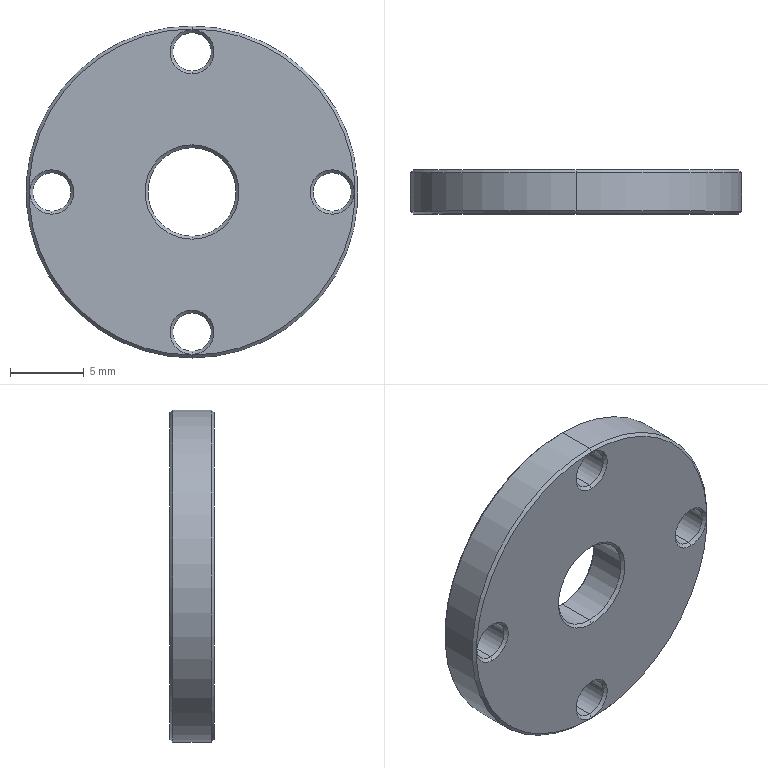Part | SolidWorks | features Chamfer 1, Extrusion 1 | 1 solid | 38 faces | box 22.5 x 3 x 22.5 mm | volume 1039 mm3 | cone 24 | cylinder 12 | plane 2 | commonest cylinder face diameters 2.6 x8 6 x2 22.5 x2
STEP:
#1=CARTESIAN_POINT('',(0.,2.8,8.2));
#2=VERTEX_POINT('',#1);
#3=CARTESIAN_POINT('',(0.,2.8,10.8));
#4=VERTEX_POINT('',#3);
#5=CARTESIAN_POINT('',(0.,2.8,9.5));
#6=DIRECTION('',(0.,1.,0.));
#7=DIRECTION('',(0.,0.,1.));
#8=AXIS2_PLACEMENT_3D('',#5,#6,#7);
#9=CIRCLE('',#8,1.3);
#10=EDGE_CURVE('',#2,#4,#9,.T.);
#11=ORIENTED_EDGE('',*,*,#10,.F.);
#12=CARTESIAN_POINT('',(0.,3.,8.));
#13=VERTEX_POINT('',#12);
#14=CARTESIAN_POINT('',(0.,2.8,8.2));
#15=DIRECTION('',(0.,0.7071,-0.7071));
#16=VECTOR('',#15,1000.);
#17=LINE('',#14,#16);
#18=EDGE_CURVE('',#2,#13,#17,.T.);
#19=ORIENTED_EDGE('',*,*,#18,.T.);
#20=CARTESIAN_POINT('',(0.,3.,11.));
#21=VERTEX_POINT('',#20);
#22=CARTESIAN_POINT('',(0.,3.,9.5));
#23=DIRECTION('',(0.,-1.,0.));
#24=DIRECTION('',(0.,0.,1.));
#25=AXIS2_PLACEMENT_3D('',#22,#23,#24);
#26=CIRCLE('',#25,1.5);
#27=EDGE_CURVE('',#21,#13,#26,.T.);
#28=ORIENTED_EDGE('',*,*,#27,.F.);
#29=CARTESIAN_POINT('',(0.,2.8,10.8));
#30=DIRECTION('',(0.,0.7071,0.7071));
#31=VECTOR('',#30,1000.);
#32=LINE('',#29,#31);
#33=EDGE_CURVE('',#4,#21,#32,.T.);
#34=ORIENTED_EDGE('',*,*,#33,.F.);
#35=EDGE_LOOP('',(#11,#19,#28,#34));
#36=FACE_OUTER_BOUND('',#35,.T.);
#37=CARTESIAN_POINT('',(0.,2.8,9.5));
#38=DIRECTION('',(0.,1.,0.));
#39=DIRECTION('',(0.,0.,1.));
#40=AXIS2_PLACEMENT_3D('',#37,#38,#39);
#41=CONICAL_SURFACE('',#40,1.3,0.7854);
#42=ADVANCED_FACE('',(#36),#41,.F.);
#43=CARTESIAN_POINT('',(0.,2.8,-3.));
#44=VERTEX_POINT('',#43);
#45=CARTESIAN_POINT('',(0.,2.8,3.));
#46=VERTEX_POINT('',#45);
#47=CARTESIAN_POINT('',(0.,2.8,0.));
#48=DIRECTION('',(0.,1.,0.));
#49=DIRECTION('',(0.,0.,1.));
#50=AXIS2_PLACEMENT_3D('',#47,#48,#49);
#51=CIRCLE('',#50,3.);
#52=EDGE_CURVE('',#44,#46,#51,.T.);
#53=ORIENTED_EDGE('',*,*,#52,.F.);
#54=CARTESIAN_POINT('',(0.,3.,-3.2));
#55=VERTEX_POINT('',#54);
#56=CARTESIAN_POINT('',(0.,2.8,-3.));
#57=DIRECTION('',(0.,0.7071,-0.7071));
#58=VECTOR('',#57,1000.);
#59=LINE('',#56,#58);
#60=EDGE_CURVE('',#44,#55,#59,.T.);
#61=ORIENTED_EDGE('',*,*,#60,.T.);
#62=CARTESIAN_POINT('',(0.,3.,3.2));
#63=VERTEX_POINT('',#62);
#64=CARTESIAN_POINT('',(0.,3.,0.));
#65=DIRECTION('',(0.,-1.,0.));
#66=DIRECTION('',(0.,0.,1.));
#67=AXIS2_PLACEMENT_3D('',#64,#65,#66);
#68=CIRCLE('',#67,3.2);
#69=EDGE_CURVE('',#63,#55,#68,.T.);
#70=ORIENTED_EDGE('',*,*,#69,.F.);
#71=CARTESIAN_POINT('',(0.,2.8,3.));
#72=DIRECTION('',(0.,0.7071,0.7071));
#73=VECTOR('',#72,1000.);
#74=LINE('',#71,#73);
#75=EDGE_CURVE('',#46,#63,#74,.T.);
#76=ORIENTED_EDGE('',*,*,#75,.F.);
#77=EDGE_LOOP('',(#53,#61,#70,#76));
#78=FACE_OUTER_BOUND('',#77,.T.);
#79=CARTESIAN_POINT('',(0.,2.8,0.));
#80=DIRECTION('',(0.,1.,0.));
#81=DIRECTION('',(0.,0.,1.));
#82=AXIS2_PLACEMENT_3D('',#79,#80,#81);
#83=CONICAL_SURFACE('',#82,3.,0.7854);
#84=ADVANCED_FACE('',(#78),#83,.F.);
#85=CARTESIAN_POINT('',(0.,3.,11.05));
#86=VERTEX_POINT('',#85);
#87=CARTESIAN_POINT('',(0.,3.,-11.05));
#88=VERTEX_POINT('',#87);
#89=CARTESIAN_POINT('',(0.,3.,0.));
#90=DIRECTION('',(0.,1.,0.));
#91=DIRECTION('',(0.,0.,1.));
#92=AXIS2_PLACEMENT_3D('',#89,#90,#91);
#93=CIRCLE('',#92,11.05);
#94=EDGE_CURVE('',#86,#88,#93,.T.);
#95=ORIENTED_EDGE('',*,*,#94,.F.);
#96=CARTESIAN_POINT('',(0.,2.8,11.25));
#97=VERTEX_POINT('',#96);
#98=CARTESIAN_POINT('',(0.,3.,11.05));
#99=DIRECTION('',(0.,-0.7071,0.7071));
#100=VECTOR('',#99,1000.);
#101=LINE('',#98,#100);
#102=EDGE_CURVE('',#86,#97,#101,.T.);
#103=ORIENTED_EDGE('',*,*,#102,.T.);
#104=CARTESIAN_POINT('',(0.,2.8,-11.25));
#105=VERTEX_POINT('',#104);
#106=CARTESIAN_POINT('',(0.,2.8,0.));
#107=DIRECTION('',(0.,-1.,0.));
#108=DIRECTION('',(0.,0.,1.));
#109=AXIS2_PLACEMENT_3D('',#106,#107,#108);
#110=CIRCLE('',#109,11.25);
#111=EDGE_CURVE('',#105,#97,#110,.T.);
#112=ORIENTED_EDGE('',*,*,#111,.F.);
#113=CARTESIAN_POINT('',(0.,3.,-11.05));
#114=DIRECTION('',(0.,-0.7071,-0.7071));
#115=VECTOR('',#114,1000.);
#116=LINE('',#113,#115);
#117=EDGE_CURVE('',#88,#105,#116,.T.);
#118=ORIENTED_EDGE('',*,*,#117,.F.);
#119=EDGE_LOOP('',(#95,#103,#112,#118));
#120=FACE_OUTER_BOUND('',#119,.T.);
#121=CARTESIAN_POINT('',(0.,3.,0.));
#122=DIRECTION('',(0.,-1.,0.));
#123=DIRECTION('',(0.,0.,-1.));
#124=AXIS2_PLACEMENT_3D('',#121,#122,#123);
#125=CONICAL_SURFACE('',#124,11.05,0.7854);
#126=ADVANCED_FACE('',(#120),#125,.T.);
#127=CARTESIAN_POINT('',(0.,2.8,-10.8));
#128=VERTEX_POINT('',#127);
#129=CARTESIAN_POINT('',(0.,2.8,-8.2));
#130=VERTEX_POINT('',#129);
#131=CARTESIAN_POINT('',(0.,2.8,-9.5));
#132=DIRECTION('',(0.,1.,0.));
#133=DIRECTION('',(0.,0.,1.));
#134=AXIS2_PLACEMENT_3D('',#131,#132,#133);
#135=CIRCLE('',#134,1.3);
#136=EDGE_CURVE('',#128,#130,#135,.T.);
#137=ORIENTED_EDGE('',*,*,#136,.F.);
#138=CARTESIAN_POINT('',(0.,3.,-11.));
#139=VERTEX_POINT('',#138);
#140=CARTESIAN_POINT('',(0.,2.8,-10.8));
#141=DIRECTION('',(0.,0.7071,-0.7071));
#142=VECTOR('',#141,1000.);
#143=LINE('',#140,#142);
#144=EDGE_CURVE('',#128,#139,#143,.T.);
#145=ORIENTED_EDGE('',*,*,#144,.T.);
#146=CARTESIAN_POINT('',(0.,3.,-8.));
#147=VERTEX_POINT('',#146);
#148=CARTESIAN_POINT('',(0.,3.,-9.5));
#149=DIRECTION('',(0.,-1.,0.));
#150=DIRECTION('',(0.,0.,1.));
#151=AXIS2_PLACEMENT_3D('',#148,#149,#150);
#152=CIRCLE('',#151,1.5);
#153=EDGE_CURVE('',#147,#139,#152,.T.);
#154=ORIENTED_EDGE('',*,*,#153,.F.);
#155=CARTESIAN_POINT('',(0.,2.8,-8.2));
#156=DIRECTION('',(0.,0.7071,0.7071));
#157=VECTOR('',#156,1000.);
#158=LINE('',#155,#157);
#159=EDGE_CURVE('',#130,#147,#158,.T.);
#160=ORIENTED_EDGE('',*,*,#159,.F.);
#161=EDGE_LOOP('',(#137,#145,#154,#160));
#162=FACE_OUTER_BOUND('',#161,.T.);
#163=CARTESIAN_POINT('',(0.,2.8,-9.5));
#164=DIRECTION('',(0.,1.,0.));
#165=DIRECTION('',(0.,0.,1.));
#166=AXIS2_PLACEMENT_3D('',#163,#164,#165);
#167=CONICAL_SURFACE('',#166,1.3,0.7854);
#168=ADVANCED_FACE('',(#162),#167,.F.);
#169=CARTESIAN_POINT('',(9.5,2.8,-1.3));
#170=VERTEX_POINT('',#169);
#171=CARTESIAN_POINT('',(9.5,2.8,1.3));
#172=VERTEX_POINT('',#171);
#173=CARTESIAN_POINT('',(9.5,2.8,0.));
#174=DIRECTION('',(0.,1.,0.));
#175=DIRECTION('',(0.,0.,1.));
#176=AXIS2_PLACEMENT_3D('',#173,#174,#175);
#177=CIRCLE('',#176,1.3);
#178=EDGE_CURVE('',#170,#172,#177,.T.);
#179=ORIENTED_EDGE('',*,*,#178,.F.);
#180=CARTESIAN_POINT('',(9.5,3.,-1.5));
#181=VERTEX_POINT('',#180);
#182=CARTESIAN_POINT('',(9.5,2.8,-1.3));
#183=DIRECTION('',(0.,0.7071,-0.7071));
#184=VECTOR('',#183,1000.);
#185=LINE('',#182,#184);
#186=EDGE_CURVE('',#170,#181,#185,.T.);
#187=ORIENTED_EDGE('',*,*,#186,.T.);
#188=CARTESIAN_POINT('',(9.5,3.,1.5));
#189=VERTEX_POINT('',#188);
#190=CARTESIAN_POINT('',(9.5,3.,0.));
#191=DIRECTION('',(0.,-1.,0.));
#192=DIRECTION('',(0.,0.,1.));
#193=AXIS2_PLACEMENT_3D('',#190,#191,#192);
#194=CIRCLE('',#193,1.5);
#195=EDGE_CURVE('',#189,#181,#194,.T.);
#196=ORIENTED_EDGE('',*,*,#195,.F.);
#197=CARTESIAN_POINT('',(9.5,2.8,1.3));
#198=DIRECTION('',(0.,0.7071,0.7071));
#199=VECTOR('',#198,1000.);
#200=LINE('',#197,#199);
#201=EDGE_CURVE('',#172,#189,#200,.T.);
#202=ORIENTED_EDGE('',*,*,#201,.F.);
#203=EDGE_LOOP('',(#179,#187,#196,#202));
#204=FACE_OUTER_BOUND('',#203,.T.);
#205=CARTESIAN_POINT('',(9.5,2.8,0.));
#206=DIRECTION('',(0.,1.,0.));
#207=DIRECTION('',(0.,0.,1.));
#208=AXIS2_PLACEMENT_3D('',#205,#206,#207);
#209=CONICAL_SURFACE('',#208,1.3,0.7854);
#210=ADVANCED_FACE('',(#204),#209,.F.);
#211=CARTESIAN_POINT('',(-9.5,2.8,-1.3));
#212=VERTEX_POINT('',#211);
#213=CARTESIAN_POINT('',(-9.5,2.8,1.3));
#214=VERTEX_POINT('',#213);
#215=CARTESIAN_POINT('',(-9.5,2.8,0.));
#216=DIRECTION('',(0.,1.,0.));
#217=DIRECTION('',(0.,0.,1.));
#218=AXIS2_PLACEMENT_3D('',#215,#216,#217);
#219=CIRCLE('',#218,1.3);
#220=EDGE_CURVE('',#212,#214,#219,.T.);
#221=ORIENTED_EDGE('',*,*,#220,.F.);
#222=CARTESIAN_POINT('',(-9.5,3.,-1.5));
#223=VERTEX_POINT('',#222);
#224=CARTESIAN_POINT('',(-9.5,2.8,-1.3));
#225=DIRECTION('',(0.,0.7071,-0.7071));
#226=VECTOR('',#225,1000.);
#227=LINE('',#224,#226);
#228=EDGE_CURVE('',#212,#223,#227,.T.);
#229=ORIENTED_EDGE('',*,*,#228,.T.);
#230=CARTESIAN_POINT('',(-9.5,3.,1.5));
#231=VERTEX_POINT('',#230);
#232=CARTESIAN_POINT('',(-9.5,3.,0.));
#233=DIRECTION('',(0.,-1.,0.));
#234=DIRECTION('',(0.,0.,1.));
#235=AXIS2_PLACEMENT_3D('',#232,#233,#234);
#236=CIRCLE('',#235,1.5);
#237=EDGE_CURVE('',#231,#223,#236,.T.);
#238=ORIENTED_EDGE('',*,*,#237,.F.);
#239=CARTESIAN_POINT('',(-9.5,2.8,1.3));
#240=DIRECTION('',(0.,0.7071,0.7071));
#241=VECTOR('',#240,1000.);
#242=LINE('',#239,#241);
#243=EDGE_CURVE('',#214,#231,#242,.T.);
#244=ORIENTED_EDGE('',*,*,#243,.F.);
#245=EDGE_LOOP('',(#221,#229,#238,#244));
#246=FACE_OUTER_BOUND('',#245,.T.);
#247=CARTESIAN_POINT('',(-9.5,2.8,0.));
#248=DIRECTION('',(0.,1.,0.));
#249=DIRECTION('',(0.,0.,1.));
#250=AXIS2_PLACEMENT_3D('',#247,#248,#249);
#251=CONICAL_SURFACE('',#250,1.3,0.7854);
#252=ADVANCED_FACE('',(#246),#251,.F.);
#253=CARTESIAN_POINT('',(0.,0.2,10.8));
#254=VERTEX_POINT('',#253);
#255=CARTESIAN_POINT('',(0.,0.2,8.2));
#256=VERTEX_POINT('',#255);
#257=CARTESIAN_POINT('',(0.,0.2,9.5));
#258=DIRECTION('',(0.,-1.,0.));
#259=DIRECTION('',(0.,0.,1.));
#260=AXIS2_PLACEMENT_3D('',#257,#258,#259);
#261=CIRCLE('',#260,1.3);
#262=EDGE_CURVE('',#254,#256,#261,.T.);
#263=ORIENTED_EDGE('',*,*,#262,.F.);
#264=CARTESIAN_POINT('',(0.,0.,11.));
#265=VERTEX_POINT('',#264);
#266=CARTESIAN_POINT('',(0.,0.,11.));
#267=DIRECTION('',(0.,-0.7071,0.7071));
#268=VECTOR('',#267,1000.);
#269=LINE('',#266,#268);
#270=EDGE_CURVE('',#254,#265,#269,.T.);
#271=ORIENTED_EDGE('',*,*,#270,.T.);
#272=CARTESIAN_POINT('',(0.,0.,8.));
#273=VERTEX_POINT('',#272);
#274=CARTESIAN_POINT('',(0.,0.,9.5));
#275=DIRECTION('',(0.,1.,0.));
#276=DIRECTION('',(0.,0.,1.));
#277=AXIS2_PLACEMENT_3D('',#274,#275,#276);
#278=CIRCLE('',#277,1.5);
#279=EDGE_CURVE('',#273,#265,#278,.T.);
#280=ORIENTED_EDGE('',*,*,#279,.F.);
#281=CARTESIAN_POINT('',(0.,0.,8.));
#282=DIRECTION('',(0.,-0.7071,-0.7071));
#283=VECTOR('',#282,1000.);
#284=LINE('',#281,#283);
#285=EDGE_CURVE('',#256,#273,#284,.T.);
#286=ORIENTED_EDGE('',*,*,#285,.F.);
#287=EDGE_LOOP('',(#263,#271,#280,#286));
#288=FACE_OUTER_BOUND('',#287,.T.);
#289=CARTESIAN_POINT('',(0.,0.,9.5));
#290=DIRECTION('',(0.,-1.,0.));
#291=DIRECTION('',(0.,0.,-1.));
#292=AXIS2_PLACEMENT_3D('',#289,#290,#291);
#293=CONICAL_SURFACE('',#292,1.5,0.7854);
#294=ADVANCED_FACE('',(#288),#293,.F.);
#295=CARTESIAN_POINT('',(0.,0.2,3.));
#296=VERTEX_POINT('',#295);
#297=CARTESIAN_POINT('',(0.,0.2,-3.));
#298=VERTEX_POINT('',#297);
#299=CARTESIAN_POINT('',(0.,0.2,0.));
#300=DIRECTION('',(0.,-1.,0.));
#301=DIRECTION('',(0.,0.,1.));
#302=AXIS2_PLACEMENT_3D('',#299,#300,#301);
#303=CIRCLE('',#302,3.);
#304=EDGE_CURVE('',#296,#298,#303,.T.);
#305=ORIENTED_EDGE('',*,*,#304,.F.);
#306=CARTESIAN_POINT('',(0.,0.,3.2));
#307=VERTEX_POINT('',#306);
#308=CARTESIAN_POINT('',(0.,0.,3.2));
#309=DIRECTION('',(0.,-0.7071,0.7071));
#310=VECTOR('',#309,1000.);
#311=LINE('',#308,#310);
#312=EDGE_CURVE('',#296,#307,#311,.T.);
#313=ORIENTED_EDGE('',*,*,#312,.T.);
#314=CARTESIAN_POINT('',(0.,0.,-3.2));
#315=VERTEX_POINT('',#314);
#316=CARTESIAN_POINT('',(0.,0.,0.));
#317=DIRECTION('',(0.,1.,0.));
#318=DIRECTION('',(0.,0.,1.));
#319=AXIS2_PLACEMENT_3D('',#316,#317,#318);
#320=CIRCLE('',#319,3.2);
#321=EDGE_CURVE('',#315,#307,#320,.T.);
#322=ORIENTED_EDGE('',*,*,#321,.F.);
#323=CARTESIAN_POINT('',(0.,0.,-3.2));
#324=DIRECTION('',(0.,-0.7071,-0.7071));
#325=VECTOR('',#324,1000.);
#326=LINE('',#323,#325);
#327=EDGE_CURVE('',#298,#315,#326,.T.);
#328=ORIENTED_EDGE('',*,*,#327,.F.);
#329=EDGE_LOOP('',(#305,#313,#322,#328));
#330=FACE_OUTER_BOUND('',#329,.T.);
#331=CARTESIAN_POINT('',(0.,0.,0.));
#332=DIRECTION('',(0.,-1.,0.));
#333=DIRECTION('',(0.,0.,-1.));
#334=AXIS2_PLACEMENT_3D('',#331,#332,#333);
#335=CONICAL_SURFACE('',#334,3.2,0.7854);
#336=ADVANCED_FACE('',(#330),#335,.F.);
#337=CARTESIAN_POINT('',(0.,0.,-11.05));
#338=VERTEX_POINT('',#337);
#339=CARTESIAN_POINT('',(0.,0.,11.05));
#340=VERTEX_POINT('',#339);
#341=CARTESIAN_POINT('',(0.,0.,0.));
#342=DIRECTION('',(0.,-1.,0.));
#343=DIRECTION('',(0.,0.,1.));
#344=AXIS2_PLACEMENT_3D('',#341,#342,#343);
#345=CIRCLE('',#344,11.05);
#346=EDGE_CURVE('',#338,#340,#345,.T.);
#347=ORIENTED_EDGE('',*,*,#346,.F.);
#348=CARTESIAN_POINT('',(0.,0.2,-11.25));
#349=VERTEX_POINT('',#348);
#350=CARTESIAN_POINT('',(0.,0.2,-11.25));
#351=DIRECTION('',(0.,0.7071,-0.7071));
#352=VECTOR('',#351,1000.);
#353=LINE('',#350,#352);
#354=EDGE_CURVE('',#338,#349,#353,.T.);
#355=ORIENTED_EDGE('',*,*,#354,.T.);
#356=CARTESIAN_POINT('',(0.,0.2,11.25));
#357=VERTEX_POINT('',#356);
#358=CARTESIAN_POINT('',(0.,0.2,0.));
#359=DIRECTION('',(0.,1.,0.));
#360=DIRECTION('',(0.,0.,1.));
#361=AXIS2_PLACEMENT_3D('',#358,#359,#360);
#362=CIRCLE('',#361,11.25);
#363=EDGE_CURVE('',#357,#349,#362,.T.);
#364=ORIENTED_EDGE('',*,*,#363,.F.);
#365=CARTESIAN_POINT('',(0.,0.2,11.25));
#366=DIRECTION('',(0.,0.7071,0.7071));
#367=VECTOR('',#366,1000.);
#368=LINE('',#365,#367);
#369=EDGE_CURVE('',#340,#357,#368,.T.);
#370=ORIENTED_EDGE('',*,*,#369,.F.);
#371=EDGE_LOOP('',(#347,#355,#364,#370));
#372=FACE_OUTER_BOUND('',#371,.T.);
#373=CARTESIAN_POINT('',(0.,0.2,0.));
#374=DIRECTION('',(0.,1.,0.));
#375=DIRECTION('',(0.,0.,1.));
#376=AXIS2_PLACEMENT_3D('',#373,#374,#375);
#377=CONICAL_SURFACE('',#376,11.25,0.7854);
#378=ADVANCED_FACE('',(#372),#377,.T.);
#379=CARTESIAN_POINT('',(0.,0.2,-8.2));
#380=VERTEX_POINT('',#379);
#381=CARTESIAN_POINT('',(0.,0.2,-10.8));
#382=VERTEX_POINT('',#381);
#383=CARTESIAN_POINT('',(0.,0.2,-9.5));
#384=DIRECTION('',(0.,-1.,0.));
#385=DIRECTION('',(0.,0.,1.));
#386=AXIS2_PLACEMENT_3D('',#383,#384,#385);
#387=CIRCLE('',#386,1.3);
#388=EDGE_CURVE('',#380,#382,#387,.T.);
#389=ORIENTED_EDGE('',*,*,#388,.F.);
#390=CARTESIAN_POINT('',(0.,0.,-8.));
#391=VERTEX_POINT('',#390);
#392=CARTESIAN_POINT('',(0.,0.,-8.));
#393=DIRECTION('',(0.,-0.7071,0.7071));
#394=VECTOR('',#393,1000.);
#395=LINE('',#392,#394);
#396=EDGE_CURVE('',#380,#391,#395,.T.);
#397=ORIENTED_EDGE('',*,*,#396,.T.);
#398=CARTESIAN_POINT('',(0.,0.,-11.));
#399=VERTEX_POINT('',#398);
#400=CARTESIAN_POINT('',(0.,0.,-9.5));
#401=DIRECTION('',(0.,1.,0.));
#402=DIRECTION('',(0.,0.,1.));
#403=AXIS2_PLACEMENT_3D('',#400,#401,#402);
#404=CIRCLE('',#403,1.5);
#405=EDGE_CURVE('',#399,#391,#404,.T.);
#406=ORIENTED_EDGE('',*,*,#405,.F.);
#407=CARTESIAN_POINT('',(0.,0.,-11.));
#408=DIRECTION('',(0.,-0.7071,-0.7071));
#409=VECTOR('',#408,1000.);
#410=LINE('',#407,#409);
#411=EDGE_CURVE('',#382,#399,#410,.T.);
#412=ORIENTED_EDGE('',*,*,#411,.F.);
#413=EDGE_LOOP('',(#389,#397,#406,#412));
#414=FACE_OUTER_BOUND('',#413,.T.);
#415=CARTESIAN_POINT('',(0.,0.,-9.5));
#416=DIRECTION('',(0.,-1.,0.));
#417=DIRECTION('',(0.,0.,-1.));
#418=AXIS2_PLACEMENT_3D('',#415,#416,#417);
#419=CONICAL_SURFACE('',#418,1.5,0.7854);
#420=ADVANCED_FACE('',(#414),#419,.F.);
#421=CARTESIAN_POINT('',(9.5,0.2,1.3));
#422=VERTEX_POINT('',#421);
#423=CARTESIAN_POINT('',(9.5,0.2,-1.3));
#424=VERTEX_POINT('',#423);
#425=CARTESIAN_POINT('',(9.5,0.2,0.));
#426=DIRECTION('',(0.,-1.,0.));
#427=DIRECTION('',(0.,0.,1.));
#428=AXIS2_PLACEMENT_3D('',#425,#426,#427);
#429=CIRCLE('',#428,1.3);
#430=EDGE_CURVE('',#422,#424,#429,.T.);
#431=ORIENTED_EDGE('',*,*,#430,.F.);
#432=CARTESIAN_POINT('',(9.5,0.,1.5));
#433=VERTEX_POINT('',#432);
#434=CARTESIAN_POINT('',(9.5,0.,1.5));
#435=DIRECTION('',(0.,-0.7071,0.7071));
#436=VECTOR('',#435,1000.);
#437=LINE('',#434,#436);
#438=EDGE_CURVE('',#422,#433,#437,.T.);
#439=ORIENTED_EDGE('',*,*,#438,.T.);
#440=CARTESIAN_POINT('',(9.5,0.,-1.5));
#441=VERTEX_POINT('',#440);
#442=CARTESIAN_POINT('',(9.5,0.,0.));
#443=DIRECTION('',(0.,1.,0.));
#444=DIRECTION('',(0.,0.,1.));
#445=AXIS2_PLACEMENT_3D('',#442,#443,#444);
#446=CIRCLE('',#445,1.5);
#447=EDGE_CURVE('',#441,#433,#446,.T.);
#448=ORIENTED_EDGE('',*,*,#447,.F.);
#449=CARTESIAN_POINT('',(9.5,0.,-1.5));
#450=DIRECTION('',(0.,-0.7071,-0.7071));
#451=VECTOR('',#450,1000.);
#452=LINE('',#449,#451);
#453=EDGE_CURVE('',#424,#441,#452,.T.);
#454=ORIENTED_EDGE('',*,*,#453,.F.);
#455=EDGE_LOOP('',(#431,#439,#448,#454));
#456=FACE_OUTER_BOUND('',#455,.T.);
#457=CARTESIAN_POINT('',(9.5,0.,0.));
#458=DIRECTION('',(0.,-1.,0.));
#459=DIRECTION('',(0.,0.,-1.));
#460=AXIS2_PLACEMENT_3D('',#457,#458,#459);
#461=CONICAL_SURFACE('',#460,1.5,0.7854);
#462=ADVANCED_FACE('',(#456),#461,.F.);
#463=CARTESIAN_POINT('',(-9.5,0.2,1.3));
#464=VERTEX_POINT('',#463);
#465=CARTESIAN_POINT('',(-9.5,0.2,-1.3));
#466=VERTEX_POINT('',#465);
#467=CARTESIAN_POINT('',(-9.5,0.2,0.));
#468=DIRECTION('',(0.,-1.,0.));
#469=DIRECTION('',(0.,0.,1.));
#470=AXIS2_PLACEMENT_3D('',#467,#468,#469);
#471=CIRCLE('',#470,1.3);
#472=EDGE_CURVE('',#464,#466,#471,.T.);
#473=ORIENTED_EDGE('',*,*,#472,.F.);
#474=CARTESIAN_POINT('',(-9.5,0.,1.5));
#475=VERTEX_POINT('',#474);
#476=CARTESIAN_POINT('',(-9.5,0.,1.5));
#477=DIRECTION('',(0.,-0.7071,0.7071));
#478=VECTOR('',#477,1000.);
#479=LINE('',#476,#478);
#480=EDGE_CURVE('',#464,#475,#479,.T.);
#481=ORIENTED_EDGE('',*,*,#480,.T.);
#482=CARTESIAN_POINT('',(-9.5,0.,-1.5));
#483=VERTEX_POINT('',#482);
#484=CARTESIAN_POINT('',(-9.5,0.,0.));
#485=DIRECTION('',(0.,1.,0.));
#486=DIRECTION('',(0.,0.,1.));
#487=AXIS2_PLACEMENT_3D('',#484,#485,#486);
#488=CIRCLE('',#487,1.5);
#489=EDGE_CURVE('',#483,#475,#488,.T.);
#490=ORIENTED_EDGE('',*,*,#489,.F.);
#491=CARTESIAN_POINT('',(-9.5,0.,-1.5));
#492=DIRECTION('',(0.,-0.7071,-0.7071));
#493=VECTOR('',#492,1000.);
#494=LINE('',#491,#493);
#495=EDGE_CURVE('',#466,#483,#494,.T.);
#496=ORIENTED_EDGE('',*,*,#495,.F.);
#497=EDGE_LOOP('',(#473,#481,#490,#496));
#498=FACE_OUTER_BOUND('',#497,.T.);
#499=CARTESIAN_POINT('',(-9.5,0.,0.));
#500=DIRECTION('',(0.,-1.,0.));
#501=DIRECTION('',(0.,0.,-1.));
#502=AXIS2_PLACEMENT_3D('',#499,#500,#501);
#503=CONICAL_SURFACE('',#502,1.5,0.7854);
#504=ADVANCED_FACE('',(#498),#503,.F.);
#505=ORIENTED_EDGE('',*,*,#220,.T.);
#506=CARTESIAN_POINT('',(-9.5,3.,1.3));
#507=DIRECTION('',(0.,-1.,0.));
#508=VECTOR('',#507,1000.);
#509=LINE('',#506,#508);
#510=EDGE_CURVE('',#214,#464,#509,.T.);
#511=ORIENTED_EDGE('',*,*,#510,.T.);
#512=ORIENTED_EDGE('',*,*,#472,.T.);
#513=CARTESIAN_POINT('',(-9.5,3.,-1.3));
#514=DIRECTION('',(0.,-1.,0.));
#515=VECTOR('',#514,1000.);
#516=LINE('',#513,#515);
#517=EDGE_CURVE('',#212,#466,#516,.T.);
#518=ORIENTED_EDGE('',*,*,#517,.F.);
#519=EDGE_LOOP('',(#505,#511,#512,#518));
#520=FACE_OUTER_BOUND('',#519,.T.);
#521=CARTESIAN_POINT('',(-9.5,3.,0.));
#522=DIRECTION('',(0.,-1.,0.));
#523=DIRECTION('',(0.,0.,-1.));
#524=AXIS2_PLACEMENT_3D('',#521,#522,#523);
#525=CYLINDRICAL_SURFACE('',#524,1.3);
#526=ADVANCED_FACE('',(#520),#525,.F.);
#527=ORIENTED_EDGE('',*,*,#10,.T.);
#528=CARTESIAN_POINT('',(0.,3.,10.8));
#529=DIRECTION('',(0.,-1.,0.));
#530=VECTOR('',#529,1000.);
#531=LINE('',#528,#530);
#532=EDGE_CURVE('',#4,#254,#531,.T.);
#533=ORIENTED_EDGE('',*,*,#532,.T.);
#534=ORIENTED_EDGE('',*,*,#262,.T.);
#535=CARTESIAN_POINT('',(0.,3.,8.2));
#536=DIRECTION('',(0.,-1.,0.));
#537=VECTOR('',#536,1000.);
#538=LINE('',#535,#537);
#539=EDGE_CURVE('',#2,#256,#538,.T.);
#540=ORIENTED_EDGE('',*,*,#539,.F.);
#541=EDGE_LOOP('',(#527,#533,#534,#540));
#542=FACE_OUTER_BOUND('',#541,.T.);
#543=CARTESIAN_POINT('',(0.,3.,9.5));
#544=DIRECTION('',(0.,-1.,0.));
#545=DIRECTION('',(0.,0.,-1.));
#546=AXIS2_PLACEMENT_3D('',#543,#544,#545);
#547=CYLINDRICAL_SURFACE('',#546,1.3);
#548=ADVANCED_FACE('',(#542),#547,.F.);
#549=ORIENTED_EDGE('',*,*,#178,.T.);
#550=CARTESIAN_POINT('',(9.5,3.,1.3));
#551=DIRECTION('',(0.,-1.,0.));
#552=VECTOR('',#551,1000.);
#553=LINE('',#550,#552);
#554=EDGE_CURVE('',#172,#422,#553,.T.);
#555=ORIENTED_EDGE('',*,*,#554,.T.);
#556=ORIENTED_EDGE('',*,*,#430,.T.);
#557=CARTESIAN_POINT('',(9.5,3.,-1.3));
#558=DIRECTION('',(0.,-1.,0.));
#559=VECTOR('',#558,1000.);
#560=LINE('',#557,#559);
#561=EDGE_CURVE('',#170,#424,#560,.T.);
#562=ORIENTED_EDGE('',*,*,#561,.F.);
#563=EDGE_LOOP('',(#549,#555,#556,#562));
#564=FACE_OUTER_BOUND('',#563,.T.);
#565=CARTESIAN_POINT('',(9.5,3.,0.));
#566=DIRECTION('',(0.,-1.,0.));
#567=DIRECTION('',(0.,0.,-1.));
#568=AXIS2_PLACEMENT_3D('',#565,#566,#567);
#569=CYLINDRICAL_SURFACE('',#568,1.3);
#570=ADVANCED_FACE('',(#564),#569,.F.);
#571=ORIENTED_EDGE('',*,*,#52,.T.);
#572=CARTESIAN_POINT('',(0.,3.,3.));
#573=DIRECTION('',(0.,-1.,0.));
#574=VECTOR('',#573,1000.);
#575=LINE('',#572,#574);
#576=EDGE_CURVE('',#46,#296,#575,.T.);
#577=ORIENTED_EDGE('',*,*,#576,.T.);
#578=ORIENTED_EDGE('',*,*,#304,.T.);
#579=CARTESIAN_POINT('',(0.,3.,-3.));
#580=DIRECTION('',(0.,-1.,0.));
#581=VECTOR('',#580,1000.);
#582=LINE('',#579,#581);
#583=EDGE_CURVE('',#44,#298,#582,.T.);
#584=ORIENTED_EDGE('',*,*,#583,.F.);
#585=EDGE_LOOP('',(#571,#577,#578,#584));
#586=FACE_OUTER_BOUND('',#585,.T.);
#587=CARTESIAN_POINT('',(0.,3.,0.));
#588=DIRECTION('',(0.,-1.,0.));
#589=DIRECTION('',(0.,0.,-1.));
#590=AXIS2_PLACEMENT_3D('',#587,#588,#589);
#591=CYLINDRICAL_SURFACE('',#590,3.);
#592=ADVANCED_FACE('',(#586),#591,.F.);
#593=ORIENTED_EDGE('',*,*,#136,.T.);
#594=CARTESIAN_POINT('',(0.,3.,-8.2));
#595=DIRECTION('',(0.,-1.,0.));
#596=VECTOR('',#595,1000.);
#597=LINE('',#594,#596);
#598=EDGE_CURVE('',#130,#380,#597,.T.);
#599=ORIENTED_EDGE('',*,*,#598,.T.);
#600=ORIENTED_EDGE('',*,*,#388,.T.);
#601=CARTESIAN_POINT('',(0.,3.,-10.8));
#602=DIRECTION('',(0.,-1.,0.));
#603=VECTOR('',#602,1000.);
#604=LINE('',#601,#603);
#605=EDGE_CURVE('',#128,#382,#604,.T.);
#606=ORIENTED_EDGE('',*,*,#605,.F.);
#607=EDGE_LOOP('',(#593,#599,#600,#606));
#608=FACE_OUTER_BOUND('',#607,.T.);
#609=CARTESIAN_POINT('',(0.,3.,-9.5));
#610=DIRECTION('',(0.,-1.,0.));
#611=DIRECTION('',(0.,0.,-1.));
#612=AXIS2_PLACEMENT_3D('',#609,#610,#611);
#613=CYLINDRICAL_SURFACE('',#612,1.3);
#614=ADVANCED_FACE('',(#608),#613,.F.);
#615=ORIENTED_EDGE('',*,*,#111,.T.);
#616=CARTESIAN_POINT('',(0.,3.,11.25));
#617=DIRECTION('',(0.,-1.,0.));
#618=VECTOR('',#617,1000.);
#619=LINE('',#616,#618);
#620=EDGE_CURVE('',#97,#357,#619,.T.);
#621=ORIENTED_EDGE('',*,*,#620,.T.);
#622=ORIENTED_EDGE('',*,*,#363,.T.);
#623=CARTESIAN_POINT('',(0.,3.,-11.25));
#624=DIRECTION('',(0.,-1.,0.));
#625=VECTOR('',#624,1000.);
#626=LINE('',#623,#625);
#627=EDGE_CURVE('',#105,#349,#626,.T.);
#628=ORIENTED_EDGE('',*,*,#627,.F.);
#629=EDGE_LOOP('',(#615,#621,#622,#628));
#630=FACE_OUTER_BOUND('',#629,.T.);
#631=CARTESIAN_POINT('',(0.,3.,0.));
#632=DIRECTION('',(0.,-1.,0.));
#633=DIRECTION('',(0.,0.,-1.));
#634=AXIS2_PLACEMENT_3D('',#631,#632,#633);
#635=CYLINDRICAL_SURFACE('',#634,11.25);
#636=ADVANCED_FACE('',(#630),#635,.T.);
#637=ORIENTED_EDGE('',*,*,#237,.T.);
#638=CARTESIAN_POINT('',(-9.5,3.,0.));
#639=DIRECTION('',(0.,-1.,0.));
#640=DIRECTION('',(0.,0.,1.));
#641=AXIS2_PLACEMENT_3D('',#638,#639,#640);
#642=CIRCLE('',#641,1.5);
#643=EDGE_CURVE('',#223,#231,#642,.T.);
#644=ORIENTED_EDGE('',*,*,#643,.T.);
#645=EDGE_LOOP('',(#637,#644));
#646=FACE_BOUND('',#645,.T.);
#647=ORIENTED_EDGE('',*,*,#195,.T.);
#648=CARTESIAN_POINT('',(9.5,3.,0.));
#649=DIRECTION('',(0.,-1.,0.));
#650=DIRECTION('',(0.,0.,1.));
#651=AXIS2_PLACEMENT_3D('',#648,#649,#650);
#652=CIRCLE('',#651,1.5);
#653=EDGE_CURVE('',#181,#189,#652,.T.);
#654=ORIENTED_EDGE('',*,*,#653,.T.);
#655=EDGE_LOOP('',(#647,#654));
#656=FACE_BOUND('',#655,.T.);
#657=ORIENTED_EDGE('',*,*,#153,.T.);
#658=CARTESIAN_POINT('',(0.,3.,-9.5));
#659=DIRECTION('',(0.,-1.,0.));
#660=DIRECTION('',(0.,0.,1.));
#661=AXIS2_PLACEMENT_3D('',#658,#659,#660);
#662=CIRCLE('',#661,1.5);
#663=EDGE_CURVE('',#139,#147,#662,.T.);
#664=ORIENTED_EDGE('',*,*,#663,.T.);
#665=EDGE_LOOP('',(#657,#664));
#666=FACE_BOUND('',#665,.T.);
#667=CARTESIAN_POINT('',(0.,3.,0.));
#668=DIRECTION('',(0.,1.,0.));
#669=DIRECTION('',(0.,0.,1.));
#670=AXIS2_PLACEMENT_3D('',#667,#668,#669);
#671=CIRCLE('',#670,11.05);
#672=EDGE_CURVE('',#88,#86,#671,.T.);
#673=ORIENTED_EDGE('',*,*,#672,.T.);
#674=ORIENTED_EDGE('',*,*,#94,.T.);
#675=EDGE_LOOP('',(#673,#674));
#676=FACE_OUTER_BOUND('',#675,.T.);
#677=ORIENTED_EDGE('',*,*,#69,.T.);
#678=CARTESIAN_POINT('',(0.,3.,0.));
#679=DIRECTION('',(0.,-1.,0.));
#680=DIRECTION('',(0.,0.,1.));
#681=AXIS2_PLACEMENT_3D('',#678,#679,#680);
#682=CIRCLE('',#681,3.2);
#683=EDGE_CURVE('',#55,#63,#682,.T.);
#684=ORIENTED_EDGE('',*,*,#683,.T.);
#685=EDGE_LOOP('',(#677,#684));
#686=FACE_BOUND('',#685,.T.);
#687=ORIENTED_EDGE('',*,*,#27,.T.);
#688=CARTESIAN_POINT('',(0.,3.,9.5));
#689=DIRECTION('',(0.,-1.,0.));
#690=DIRECTION('',(0.,0.,1.));
#691=AXIS2_PLACEMENT_3D('',#688,#689,#690);
#692=CIRCLE('',#691,1.5);
#693=EDGE_CURVE('',#13,#21,#692,.T.);
#694=ORIENTED_EDGE('',*,*,#693,.T.);
#695=EDGE_LOOP('',(#687,#694));
#696=FACE_BOUND('',#695,.T.);
#697=CARTESIAN_POINT('',(0.,3.,0.));
#698=DIRECTION('',(0.,1.,0.));
#699=DIRECTION('',(0.,0.,1.));
#700=AXIS2_PLACEMENT_3D('',#697,#698,#699);
#701=PLANE('',#700);
#702=ADVANCED_FACE('',(#646,#656,#666,#676,#686,#696),#701,.T.);
#703=ORIENTED_EDGE('',*,*,#489,.T.);
#704=CARTESIAN_POINT('',(-9.5,0.,0.));
#705=DIRECTION('',(0.,1.,0.));
#706=DIRECTION('',(0.,0.,1.));
#707=AXIS2_PLACEMENT_3D('',#704,#705,#706);
#708=CIRCLE('',#707,1.5);
#709=EDGE_CURVE('',#475,#483,#708,.T.);
#710=ORIENTED_EDGE('',*,*,#709,.T.);
#711=EDGE_LOOP('',(#703,#710));
#712=FACE_BOUND('',#711,.T.);
#713=ORIENTED_EDGE('',*,*,#447,.T.);
#714=CARTESIAN_POINT('',(9.5,0.,0.));
#715=DIRECTION('',(0.,1.,0.));
#716=DIRECTION('',(0.,0.,1.));
#717=AXIS2_PLACEMENT_3D('',#714,#715,#716);
#718=CIRCLE('',#717,1.5);
#719=EDGE_CURVE('',#433,#441,#718,.T.);
#720=ORIENTED_EDGE('',*,*,#719,.T.);
#721=EDGE_LOOP('',(#713,#720));
#722=FACE_BOUND('',#721,.T.);
#723=ORIENTED_EDGE('',*,*,#405,.T.);
#724=CARTESIAN_POINT('',(0.,0.,-9.5));
#725=DIRECTION('',(0.,1.,0.));
#726=DIRECTION('',(0.,0.,1.));
#727=AXIS2_PLACEMENT_3D('',#724,#725,#726);
#728=CIRCLE('',#727,1.5);
#729=EDGE_CURVE('',#391,#399,#728,.T.);
#730=ORIENTED_EDGE('',*,*,#729,.T.);
#731=EDGE_LOOP('',(#723,#730));
#732=FACE_BOUND('',#731,.T.);
#733=CARTESIAN_POINT('',(0.,0.,0.));
#734=DIRECTION('',(0.,-1.,0.));
#735=DIRECTION('',(0.,0.,1.));
#736=AXIS2_PLACEMENT_3D('',#733,#734,#735);
#737=CIRCLE('',#736,11.05);
#738=EDGE_CURVE('',#340,#338,#737,.T.);
#739=ORIENTED_EDGE('',*,*,#738,.T.);
#740=ORIENTED_EDGE('',*,*,#346,.T.);
#741=EDGE_LOOP('',(#739,#740));
#742=FACE_OUTER_BOUND('',#741,.T.);
#743=ORIENTED_EDGE('',*,*,#321,.T.);
#744=CARTESIAN_POINT('',(0.,0.,0.));
#745=DIRECTION('',(0.,1.,0.));
#746=DIRECTION('',(0.,0.,1.));
#747=AXIS2_PLACEMENT_3D('',#744,#745,#746);
#748=CIRCLE('',#747,3.2);
#749=EDGE_CURVE('',#307,#315,#748,.T.);
#750=ORIENTED_EDGE('',*,*,#749,.T.);
#751=EDGE_LOOP('',(#743,#750));
#752=FACE_BOUND('',#751,.T.);
#753=ORIENTED_EDGE('',*,*,#279,.T.);
#754=CARTESIAN_POINT('',(0.,0.,9.5));
#755=DIRECTION('',(0.,1.,0.));
#756=DIRECTION('',(0.,0.,1.));
#757=AXIS2_PLACEMENT_3D('',#754,#755,#756);
#758=CIRCLE('',#757,1.5);
#759=EDGE_CURVE('',#265,#273,#758,.T.);
#760=ORIENTED_EDGE('',*,*,#759,.T.);
#761=EDGE_LOOP('',(#753,#760));
#762=FACE_BOUND('',#761,.T.);
#763=CARTESIAN_POINT('',(0.,0.,0.));
#764=DIRECTION('',(0.,1.,0.));
#765=DIRECTION('',(0.,0.,1.));
#766=AXIS2_PLACEMENT_3D('',#763,#764,#765);
#767=PLANE('',#766);
#768=ADVANCED_FACE('',(#712,#722,#732,#742,#752,#762),#767,.F.);
#769=ORIENTED_EDGE('',*,*,#620,.F.);
#770=CARTESIAN_POINT('',(0.,2.8,0.));
#771=DIRECTION('',(0.,-1.,0.));
#772=DIRECTION('',(0.,0.,1.));
#773=AXIS2_PLACEMENT_3D('',#770,#771,#772);
#774=CIRCLE('',#773,11.25);
#775=EDGE_CURVE('',#97,#105,#774,.T.);
#776=ORIENTED_EDGE('',*,*,#775,.T.);
#777=ORIENTED_EDGE('',*,*,#627,.T.);
#778=CARTESIAN_POINT('',(0.,0.2,0.));
#779=DIRECTION('',(0.,1.,0.));
#780=DIRECTION('',(0.,0.,1.));
#781=AXIS2_PLACEMENT_3D('',#778,#779,#780);
#782=CIRCLE('',#781,11.25);
#783=EDGE_CURVE('',#349,#357,#782,.T.);
#784=ORIENTED_EDGE('',*,*,#783,.T.);
#785=EDGE_LOOP('',(#769,#776,#777,#784));
#786=FACE_OUTER_BOUND('',#785,.T.);
#787=CARTESIAN_POINT('',(0.,3.,0.));
#788=DIRECTION('',(0.,-1.,0.));
#789=DIRECTION('',(0.,0.,-1.));
#790=AXIS2_PLACEMENT_3D('',#787,#788,#789);
#791=CYLINDRICAL_SURFACE('',#790,11.25);
#792=ADVANCED_FACE('',(#786),#791,.T.);
#793=ORIENTED_EDGE('',*,*,#598,.F.);
#794=CARTESIAN_POINT('',(0.,2.8,-9.5));
#795=DIRECTION('',(0.,1.,0.));
#796=DIRECTION('',(0.,0.,1.));
#797=AXIS2_PLACEMENT_3D('',#794,#795,#796);
#798=CIRCLE('',#797,1.3);
#799=EDGE_CURVE('',#130,#128,#798,.T.);
#800=ORIENTED_EDGE('',*,*,#799,.T.);
#801=ORIENTED_EDGE('',*,*,#605,.T.);
#802=CARTESIAN_POINT('',(0.,0.2,-9.5));
#803=DIRECTION('',(0.,-1.,0.));
#804=DIRECTION('',(0.,0.,1.));
#805=AXIS2_PLACEMENT_3D('',#802,#803,#804);
#806=CIRCLE('',#805,1.3);
#807=EDGE_CURVE('',#382,#380,#806,.T.);
#808=ORIENTED_EDGE('',*,*,#807,.T.);
#809=EDGE_LOOP('',(#793,#800,#801,#808));
#810=FACE_OUTER_BOUND('',#809,.T.);
#811=CARTESIAN_POINT('',(0.,3.,-9.5));
#812=DIRECTION('',(0.,-1.,0.));
#813=DIRECTION('',(0.,0.,-1.));
#814=AXIS2_PLACEMENT_3D('',#811,#812,#813);
#815=CYLINDRICAL_SURFACE('',#814,1.3);
#816=ADVANCED_FACE('',(#810),#815,.F.);
#817=ORIENTED_EDGE('',*,*,#576,.F.);
#818=CARTESIAN_POINT('',(0.,2.8,0.));
#819=DIRECTION('',(0.,1.,0.));
#820=DIRECTION('',(0.,0.,1.));
#821=AXIS2_PLACEMENT_3D('',#818,#819,#820);
#822=CIRCLE('',#821,3.);
#823=EDGE_CURVE('',#46,#44,#822,.T.);
#824=ORIENTED_EDGE('',*,*,#823,.T.);
#825=ORIENTED_EDGE('',*,*,#583,.T.);
#826=CARTESIAN_POINT('',(0.,0.2,0.));
#827=DIRECTION('',(0.,-1.,0.));
#828=DIRECTION('',(0.,0.,1.));
#829=AXIS2_PLACEMENT_3D('',#826,#827,#828);
#830=CIRCLE('',#829,3.);
#831=EDGE_CURVE('',#298,#296,#830,.T.);
#832=ORIENTED_EDGE('',*,*,#831,.T.);
#833=EDGE_LOOP('',(#817,#824,#825,#832));
#834=FACE_OUTER_BOUND('',#833,.T.);
#835=CARTESIAN_POINT('',(0.,3.,0.));
#836=DIRECTION('',(0.,-1.,0.));
#837=DIRECTION('',(0.,0.,-1.));
#838=AXIS2_PLACEMENT_3D('',#835,#836,#837);
#839=CYLINDRICAL_SURFACE('',#838,3.);
#840=ADVANCED_FACE('',(#834),#839,.F.);
#841=ORIENTED_EDGE('',*,*,#554,.F.);
#842=CARTESIAN_POINT('',(9.5,2.8,0.));
#843=DIRECTION('',(0.,1.,0.));
#844=DIRECTION('',(0.,0.,1.));
#845=AXIS2_PLACEMENT_3D('',#842,#843,#844);
#846=CIRCLE('',#845,1.3);
#847=EDGE_CURVE('',#172,#170,#846,.T.);
#848=ORIENTED_EDGE('',*,*,#847,.T.);
#849=ORIENTED_EDGE('',*,*,#561,.T.);
#850=CARTESIAN_POINT('',(9.5,0.2,0.));
#851=DIRECTION('',(0.,-1.,0.));
#852=DIRECTION('',(0.,0.,1.));
#853=AXIS2_PLACEMENT_3D('',#850,#851,#852);
#854=CIRCLE('',#853,1.3);
#855=EDGE_CURVE('',#424,#422,#854,.T.);
#856=ORIENTED_EDGE('',*,*,#855,.T.);
#857=EDGE_LOOP('',(#841,#848,#849,#856));
#858=FACE_OUTER_BOUND('',#857,.T.);
#859=CARTESIAN_POINT('',(9.5,3.,0.));
#860=DIRECTION('',(0.,-1.,0.));
#861=DIRECTION('',(0.,0.,-1.));
#862=AXIS2_PLACEMENT_3D('',#859,#860,#861);
#863=CYLINDRICAL_SURFACE('',#862,1.3);
#864=ADVANCED_FACE('',(#858),#863,.F.);
#865=ORIENTED_EDGE('',*,*,#532,.F.);
#866=CARTESIAN_POINT('',(0.,2.8,9.5));
#867=DIRECTION('',(0.,1.,0.));
#868=DIRECTION('',(0.,0.,1.));
#869=AXIS2_PLACEMENT_3D('',#866,#867,#868);
#870=CIRCLE('',#869,1.3);
#871=EDGE_CURVE('',#4,#2,#870,.T.);
#872=ORIENTED_EDGE('',*,*,#871,.T.);
#873=ORIENTED_EDGE('',*,*,#539,.T.);
#874=CARTESIAN_POINT('',(0.,0.2,9.5));
#875=DIRECTION('',(0.,-1.,0.));
#876=DIRECTION('',(0.,0.,1.));
#877=AXIS2_PLACEMENT_3D('',#874,#875,#876);
#878=CIRCLE('',#877,1.3);
#879=EDGE_CURVE('',#256,#254,#878,.T.);
#880=ORIENTED_EDGE('',*,*,#879,.T.);
#881=EDGE_LOOP('',(#865,#872,#873,#880));
#882=FACE_OUTER_BOUND('',#881,.T.);
#883=CARTESIAN_POINT('',(0.,3.,9.5));
#884=DIRECTION('',(0.,-1.,0.));
#885=DIRECTION('',(0.,0.,-1.));
#886=AXIS2_PLACEMENT_3D('',#883,#884,#885);
#887=CYLINDRICAL_SURFACE('',#886,1.3);
#888=ADVANCED_FACE('',(#882),#887,.F.);
#889=ORIENTED_EDGE('',*,*,#510,.F.);
#890=CARTESIAN_POINT('',(-9.5,2.8,0.));
#891=DIRECTION('',(0.,1.,0.));
#892=DIRECTION('',(0.,0.,1.));
#893=AXIS2_PLACEMENT_3D('',#890,#891,#892);
#894=CIRCLE('',#893,1.3);
#895=EDGE_CURVE('',#214,#212,#894,.T.);
#896=ORIENTED_EDGE('',*,*,#895,.T.);
#897=ORIENTED_EDGE('',*,*,#517,.T.);
#898=CARTESIAN_POINT('',(-9.5,0.2,0.));
#899=DIRECTION('',(0.,-1.,0.));
#900=DIRECTION('',(0.,0.,1.));
#901=AXIS2_PLACEMENT_3D('',#898,#899,#900);
#902=CIRCLE('',#901,1.3);
#903=EDGE_CURVE('',#466,#464,#902,.T.);
#904=ORIENTED_EDGE('',*,*,#903,.T.);
#905=EDGE_LOOP('',(#889,#896,#897,#904));
#906=FACE_OUTER_BOUND('',#905,.T.);
#907=CARTESIAN_POINT('',(-9.5,3.,0.));
#908=DIRECTION('',(0.,-1.,0.));
#909=DIRECTION('',(0.,0.,-1.));
#910=AXIS2_PLACEMENT_3D('',#907,#908,#909);
#911=CYLINDRICAL_SURFACE('',#910,1.3);
#912=ADVANCED_FACE('',(#906),#911,.F.);
#913=ORIENTED_EDGE('',*,*,#480,.F.);
#914=ORIENTED_EDGE('',*,*,#903,.F.);
#915=ORIENTED_EDGE('',*,*,#495,.T.);
#916=ORIENTED_EDGE('',*,*,#709,.F.);
#917=EDGE_LOOP('',(#913,#914,#915,#916));
#918=FACE_OUTER_BOUND('',#917,.T.);
#919=CARTESIAN_POINT('',(-9.5,0.,0.));
#920=DIRECTION('',(0.,-1.,0.));
#921=DIRECTION('',(0.,0.,-1.));
#922=AXIS2_PLACEMENT_3D('',#919,#920,#921);
#923=CONICAL_SURFACE('',#922,1.5,0.7854);
#924=ADVANCED_FACE('',(#918),#923,.F.);
#925=ORIENTED_EDGE('',*,*,#438,.F.);
#926=ORIENTED_EDGE('',*,*,#855,.F.);
#927=ORIENTED_EDGE('',*,*,#453,.T.);
#928=ORIENTED_EDGE('',*,*,#719,.F.);
#929=EDGE_LOOP('',(#925,#926,#927,#928));
#930=FACE_OUTER_BOUND('',#929,.T.);
#931=CARTESIAN_POINT('',(9.5,0.,0.));
#932=DIRECTION('',(0.,-1.,0.));
#933=DIRECTION('',(0.,0.,-1.));
#934=AXIS2_PLACEMENT_3D('',#931,#932,#933);
#935=CONICAL_SURFACE('',#934,1.5,0.7854);
#936=ADVANCED_FACE('',(#930),#935,.F.);
#937=ORIENTED_EDGE('',*,*,#396,.F.);
#938=ORIENTED_EDGE('',*,*,#807,.F.);
#939=ORIENTED_EDGE('',*,*,#411,.T.);
#940=ORIENTED_EDGE('',*,*,#729,.F.);
#941=EDGE_LOOP('',(#937,#938,#939,#940));
#942=FACE_OUTER_BOUND('',#941,.T.);
#943=CARTESIAN_POINT('',(0.,0.,-9.5));
#944=DIRECTION('',(0.,-1.,0.));
#945=DIRECTION('',(0.,0.,-1.));
#946=AXIS2_PLACEMENT_3D('',#943,#944,#945);
#947=CONICAL_SURFACE('',#946,1.5,0.7854);
#948=ADVANCED_FACE('',(#942),#947,.F.);
#949=ORIENTED_EDGE('',*,*,#354,.F.);
#950=ORIENTED_EDGE('',*,*,#738,.F.);
#951=ORIENTED_EDGE('',*,*,#369,.T.);
#952=ORIENTED_EDGE('',*,*,#783,.F.);
#953=EDGE_LOOP('',(#949,#950,#951,#952));
#954=FACE_OUTER_BOUND('',#953,.T.);
#955=CARTESIAN_POINT('',(0.,0.2,0.));
#956=DIRECTION('',(0.,1.,0.));
#957=DIRECTION('',(0.,0.,1.));
#958=AXIS2_PLACEMENT_3D('',#955,#956,#957);
#959=CONICAL_SURFACE('',#958,11.25,0.7854);
#960=ADVANCED_FACE('',(#954),#959,.T.);
#961=ORIENTED_EDGE('',*,*,#312,.F.);
#962=ORIENTED_EDGE('',*,*,#831,.F.);
#963=ORIENTED_EDGE('',*,*,#327,.T.);
#964=ORIENTED_EDGE('',*,*,#749,.F.);
#965=EDGE_LOOP('',(#961,#962,#963,#964));
#966=FACE_OUTER_BOUND('',#965,.T.);
#967=CARTESIAN_POINT('',(0.,0.,0.));
#968=DIRECTION('',(0.,-1.,0.));
#969=DIRECTION('',(0.,0.,-1.));
#970=AXIS2_PLACEMENT_3D('',#967,#968,#969);
#971=CONICAL_SURFACE('',#970,3.2,0.7854);
#972=ADVANCED_FACE('',(#966),#971,.F.);
#973=ORIENTED_EDGE('',*,*,#270,.F.);
#974=ORIENTED_EDGE('',*,*,#879,.F.);
#975=ORIENTED_EDGE('',*,*,#285,.T.);
#976=ORIENTED_EDGE('',*,*,#759,.F.);
#977=EDGE_LOOP('',(#973,#974,#975,#976));
#978=FACE_OUTER_BOUND('',#977,.T.);
#979=CARTESIAN_POINT('',(0.,0.,9.5));
#980=DIRECTION('',(0.,-1.,0.));
#981=DIRECTION('',(0.,0.,-1.));
#982=AXIS2_PLACEMENT_3D('',#979,#980,#981);
#983=CONICAL_SURFACE('',#982,1.5,0.7854);
#984=ADVANCED_FACE('',(#978),#983,.F.);
#985=ORIENTED_EDGE('',*,*,#228,.F.);
#986=ORIENTED_EDGE('',*,*,#895,.F.);
#987=ORIENTED_EDGE('',*,*,#243,.T.);
#988=ORIENTED_EDGE('',*,*,#643,.F.);
#989=EDGE_LOOP('',(#985,#986,#987,#988));
#990=FACE_OUTER_BOUND('',#989,.T.);
#991=CARTESIAN_POINT('',(-9.5,2.8,0.));
#992=DIRECTION('',(0.,1.,0.));
#993=DIRECTION('',(0.,0.,1.));
#994=AXIS2_PLACEMENT_3D('',#991,#992,#993);
#995=CONICAL_SURFACE('',#994,1.3,0.7854);
#996=ADVANCED_FACE('',(#990),#995,.F.);
#997=ORIENTED_EDGE('',*,*,#186,.F.);
#998=ORIENTED_EDGE('',*,*,#847,.F.);
#999=ORIENTED_EDGE('',*,*,#201,.T.);
#1000=ORIENTED_EDGE('',*,*,#653,.F.);
#1001=EDGE_LOOP('',(#997,#998,#999,#1000));
#1002=FACE_OUTER_BOUND('',#1001,.T.);
#1003=CARTESIAN_POINT('',(9.5,2.8,0.));
#1004=DIRECTION('',(0.,1.,0.));
#1005=DIRECTION('',(0.,0.,1.));
#1006=AXIS2_PLACEMENT_3D('',#1003,#1004,#1005);
#1007=CONICAL_SURFACE('',#1006,1.3,0.7854);
#1008=ADVANCED_FACE('',(#1002),#1007,.F.);
#1009=ORIENTED_EDGE('',*,*,#144,.F.);
#1010=ORIENTED_EDGE('',*,*,#799,.F.);
#1011=ORIENTED_EDGE('',*,*,#159,.T.);
#1012=ORIENTED_EDGE('',*,*,#663,.F.);
#1013=EDGE_LOOP('',(#1009,#1010,#1011,#1012));
#1014=FACE_OUTER_BOUND('',#1013,.T.);
#1015=CARTESIAN_POINT('',(0.,2.8,-9.5));
#1016=DIRECTION('',(0.,1.,0.));
#1017=DIRECTION('',(0.,0.,1.));
#1018=AXIS2_PLACEMENT_3D('',#1015,#1016,#1017);
#1019=CONICAL_SURFACE('',#1018,1.3,0.7854);
#1020=ADVANCED_FACE('',(#1014),#1019,.F.);
#1021=ORIENTED_EDGE('',*,*,#102,.F.);
#1022=ORIENTED_EDGE('',*,*,#672,.F.);
#1023=ORIENTED_EDGE('',*,*,#117,.T.);
#1024=ORIENTED_EDGE('',*,*,#775,.F.);
#1025=EDGE_LOOP('',(#1021,#1022,#1023,#1024));
#1026=FACE_OUTER_BOUND('',#1025,.T.);
#1027=CARTESIAN_POINT('',(0.,3.,0.));
#1028=DIRECTION('',(0.,-1.,0.));
#1029=DIRECTION('',(0.,0.,-1.));
#1030=AXIS2_PLACEMENT_3D('',#1027,#1028,#1029);
#1031=CONICAL_SURFACE('',#1030,11.05,0.7854);
#1032=ADVANCED_FACE('',(#1026),#1031,.T.);
#1033=ORIENTED_EDGE('',*,*,#60,.F.);
#1034=ORIENTED_EDGE('',*,*,#823,.F.);
#1035=ORIENTED_EDGE('',*,*,#75,.T.);
#1036=ORIENTED_EDGE('',*,*,#683,.F.);
#1037=EDGE_LOOP('',(#1033,#1034,#1035,#1036));
#1038=FACE_OUTER_BOUND('',#1037,.T.);
#1039=CARTESIAN_POINT('',(0.,2.8,0.));
#1040=DIRECTION('',(0.,1.,0.));
#1041=DIRECTION('',(0.,0.,1.));
#1042=AXIS2_PLACEMENT_3D('',#1039,#1040,#1041);
#1043=CONICAL_SURFACE('',#1042,3.,0.7854);
#1044=ADVANCED_FACE('',(#1038),#1043,.F.);
#1045=ORIENTED_EDGE('',*,*,#18,.F.);
#1046=ORIENTED_EDGE('',*,*,#871,.F.);
#1047=ORIENTED_EDGE('',*,*,#33,.T.);
#1048=ORIENTED_EDGE('',*,*,#693,.F.);
#1049=EDGE_LOOP('',(#1045,#1046,#1047,#1048));
#1050=FACE_OUTER_BOUND('',#1049,.T.);
#1051=CARTESIAN_POINT('',(0.,2.8,9.5));
#1052=DIRECTION('',(0.,1.,0.));
#1053=DIRECTION('',(0.,0.,1.));
#1054=AXIS2_PLACEMENT_3D('',#1051,#1052,#1053);
#1055=CONICAL_SURFACE('',#1054,1.3,0.7854);
#1056=ADVANCED_FACE('',(#1050),#1055,.F.);
#1057=CLOSED_SHELL('',(#42,#84,#126,#168,#210,#252,#294,#336,#378,#420,#462,#504,#526,#548,#570,#592,#614,#636,#702,#768,#792,#816,#840,#864,#888,#912,#924,#936,#948,#960,#972,#984,#996,#1008,#1020,#1032,#1044,#1056));
#1058=MANIFOLD_SOLID_BREP('',#1057);
#1059=CARTESIAN_POINT('',(0.,0.,0.));
#1060=DIRECTION('',(0.,0.,1.));
#1061=DIRECTION('',(1.,0.,0.));
#1062=AXIS2_PLACEMENT_3D('',#1059,#1060,#1061);
#1063=(LENGTH_UNIT()NAMED_UNIT(*)SI_UNIT(.MILLI.,.METRE.));
#1064=UNCERTAINTY_MEASURE_WITH_UNIT(LENGTH_MEASURE(0.00001),#1063,'','');
#1065=(NAMED_UNIT(*)PLANE_ANGLE_UNIT()SI_UNIT($,.RADIAN.));
#1066=(NAMED_UNIT(*)SI_UNIT($,.STERADIAN.)SOLID_ANGLE_UNIT());
#1067=(GEOMETRIC_REPRESENTATION_CONTEXT(3)GLOBAL_UNCERTAINTY_ASSIGNED_CONTEXT((#1064))GLOBAL_UNIT_ASSIGNED_CONTEXT((#1063,#1065,#1066))REPRESENTATION_CONTEXT('',''));
#1068=ADVANCED_BREP_SHAPE_REPRESENTATION('',(#1058,#1062),#1067);